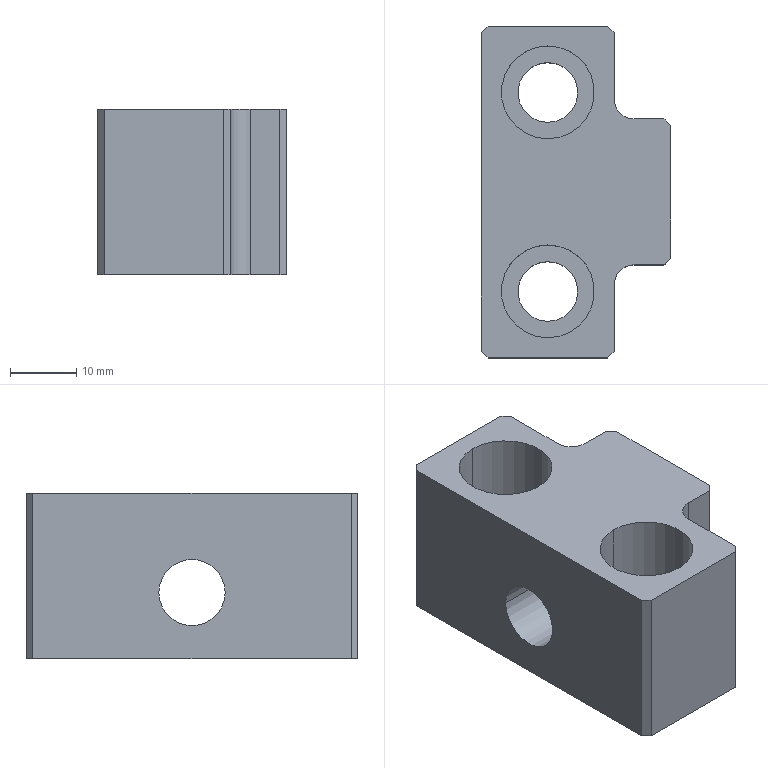Part | STEP file | J454-EBZ05-30-00-Part-1 | 1 solid | 30 faces | box 28.5 x 50 x 25 mm | volume 22471 mm3 | plane 18 | cylinder 12 | commonest cylinder face diameters 9 x4 14 x4 6 x2 10 x2
STEP:
#1=CARTESIAN_POINT('',(18.5,-5.,0.));
#2=VERTEX_POINT('',#1);
#3=CARTESIAN_POINT('',(18.5,5.,0.));
#4=VERTEX_POINT('',#3);
#5=CARTESIAN_POINT('',(18.5,0.,0.));
#6=DIRECTION('',(-1.,0.,0.));
#7=DIRECTION('',(0.,1.,0.));
#8=AXIS2_PLACEMENT_3D('',#5,#6,#7);
#9=CIRCLE('',#8,5.);
#10=EDGE_CURVE('',#2,#4,#9,.T.);
#11=ORIENTED_EDGE('',*,*,#10,.F.);
#12=CARTESIAN_POINT('',(-10.,-5.,0.));
#13=VERTEX_POINT('',#12);
#14=CARTESIAN_POINT('',(18.5,-5.,0.));
#15=DIRECTION('',(-1.,0.,0.));
#16=VECTOR('',#15,1000.);
#17=LINE('',#14,#16);
#18=EDGE_CURVE('',#2,#13,#17,.T.);
#19=ORIENTED_EDGE('',*,*,#18,.T.);
#20=CARTESIAN_POINT('',(-10.,5.,0.));
#21=VERTEX_POINT('',#20);
#22=CARTESIAN_POINT('',(-10.,0.,0.));
#23=DIRECTION('',(1.,0.,0.));
#24=DIRECTION('',(0.,-1.,0.));
#25=AXIS2_PLACEMENT_3D('',#22,#23,#24);
#26=CIRCLE('',#25,5.);
#27=EDGE_CURVE('',#21,#13,#26,.T.);
#28=ORIENTED_EDGE('',*,*,#27,.F.);
#29=CARTESIAN_POINT('',(18.5,5.,0.));
#30=DIRECTION('',(-1.,0.,0.));
#31=VECTOR('',#30,1000.);
#32=LINE('',#29,#31);
#33=EDGE_CURVE('',#4,#21,#32,.T.);
#34=ORIENTED_EDGE('',*,*,#33,.F.);
#35=EDGE_LOOP('',(#11,#19,#28,#34));
#36=FACE_OUTER_BOUND('',#35,.T.);
#37=CARTESIAN_POINT('',(18.5,0.,0.));
#38=DIRECTION('',(-1.,0.,0.));
#39=DIRECTION('',(0.,1.,0.));
#40=AXIS2_PLACEMENT_3D('',#37,#38,#39);
#41=CYLINDRICAL_SURFACE('',#40,5.);
#42=ADVANCED_FACE('',(#36),#41,.F.);
#43=CARTESIAN_POINT('',(0.,19.5,-10.));
#44=VERTEX_POINT('',#43);
#45=CARTESIAN_POINT('',(0.,10.5,-10.));
#46=VERTEX_POINT('',#45);
#47=CARTESIAN_POINT('',(0.,15.,-10.));
#48=DIRECTION('',(0.,0.,1.));
#49=DIRECTION('',(0.,-1.,0.));
#50=AXIS2_PLACEMENT_3D('',#47,#48,#49);
#51=CIRCLE('',#50,4.5);
#52=EDGE_CURVE('',#44,#46,#51,.T.);
#53=ORIENTED_EDGE('',*,*,#52,.F.);
#54=CARTESIAN_POINT('',(0.,19.5,5.));
#55=VERTEX_POINT('',#54);
#56=CARTESIAN_POINT('',(0.,19.5,15.));
#57=DIRECTION('',(0.,0.,1.));
#58=VECTOR('',#57,1000.);
#59=LINE('',#56,#58);
#60=EDGE_CURVE('',#44,#55,#59,.T.);
#61=ORIENTED_EDGE('',*,*,#60,.T.);
#62=CARTESIAN_POINT('',(0.,10.5,5.));
#63=VERTEX_POINT('',#62);
#64=CARTESIAN_POINT('',(0.,15.,5.));
#65=DIRECTION('',(0.,0.,1.));
#66=DIRECTION('',(0.,-1.,0.));
#67=AXIS2_PLACEMENT_3D('',#64,#65,#66);
#68=CIRCLE('',#67,4.5);
#69=EDGE_CURVE('',#55,#63,#68,.T.);
#70=ORIENTED_EDGE('',*,*,#69,.T.);
#71=CARTESIAN_POINT('',(0.,10.5,15.));
#72=DIRECTION('',(0.,0.,1.));
#73=VECTOR('',#72,1000.);
#74=LINE('',#71,#73);
#75=EDGE_CURVE('',#46,#63,#74,.T.);
#76=ORIENTED_EDGE('',*,*,#75,.F.);
#77=EDGE_LOOP('',(#53,#61,#70,#76));
#78=FACE_OUTER_BOUND('',#77,.T.);
#79=CARTESIAN_POINT('',(0.,15.,15.));
#80=DIRECTION('',(0.,0.,1.));
#81=DIRECTION('',(0.,-1.,0.));
#82=AXIS2_PLACEMENT_3D('',#79,#80,#81);
#83=CYLINDRICAL_SURFACE('',#82,4.5);
#84=ADVANCED_FACE('',(#78),#83,.F.);
#85=CARTESIAN_POINT('',(0.,22.,5.));
#86=VERTEX_POINT('',#85);
#87=CARTESIAN_POINT('',(0.,8.,5.));
#88=VERTEX_POINT('',#87);
#89=CARTESIAN_POINT('',(0.,15.,5.));
#90=DIRECTION('',(0.,0.,1.));
#91=DIRECTION('',(0.,-1.,0.));
#92=AXIS2_PLACEMENT_3D('',#89,#90,#91);
#93=CIRCLE('',#92,7.);
#94=EDGE_CURVE('',#86,#88,#93,.T.);
#95=ORIENTED_EDGE('',*,*,#94,.F.);
#96=CARTESIAN_POINT('',(0.,22.,15.));
#97=VERTEX_POINT('',#96);
#98=CARTESIAN_POINT('',(0.,22.,15.));
#99=DIRECTION('',(0.,0.,1.));
#100=VECTOR('',#99,1000.);
#101=LINE('',#98,#100);
#102=EDGE_CURVE('',#86,#97,#101,.T.);
#103=ORIENTED_EDGE('',*,*,#102,.T.);
#104=CARTESIAN_POINT('',(0.,8.,15.));
#105=VERTEX_POINT('',#104);
#106=CARTESIAN_POINT('',(0.,15.,15.));
#107=DIRECTION('',(0.,0.,1.));
#108=DIRECTION('',(0.,-1.,0.));
#109=AXIS2_PLACEMENT_3D('',#106,#107,#108);
#110=CIRCLE('',#109,7.);
#111=EDGE_CURVE('',#97,#105,#110,.T.);
#112=ORIENTED_EDGE('',*,*,#111,.T.);
#113=CARTESIAN_POINT('',(0.,8.,15.));
#114=DIRECTION('',(0.,0.,1.));
#115=VECTOR('',#114,1000.);
#116=LINE('',#113,#115);
#117=EDGE_CURVE('',#88,#105,#116,.T.);
#118=ORIENTED_EDGE('',*,*,#117,.F.);
#119=EDGE_LOOP('',(#95,#103,#112,#118));
#120=FACE_OUTER_BOUND('',#119,.T.);
#121=CARTESIAN_POINT('',(0.,15.,15.));
#122=DIRECTION('',(0.,0.,1.));
#123=DIRECTION('',(0.,-1.,0.));
#124=AXIS2_PLACEMENT_3D('',#121,#122,#123);
#125=CYLINDRICAL_SURFACE('',#124,7.);
#126=ADVANCED_FACE('',(#120),#125,.F.);
#127=CARTESIAN_POINT('',(0.,-10.5,-10.));
#128=VERTEX_POINT('',#127);
#129=CARTESIAN_POINT('',(0.,-19.5,-10.));
#130=VERTEX_POINT('',#129);
#131=CARTESIAN_POINT('',(0.,-15.,-10.));
#132=DIRECTION('',(0.,0.,1.));
#133=DIRECTION('',(0.,-1.,0.));
#134=AXIS2_PLACEMENT_3D('',#131,#132,#133);
#135=CIRCLE('',#134,4.5);
#136=EDGE_CURVE('',#128,#130,#135,.T.);
#137=ORIENTED_EDGE('',*,*,#136,.F.);
#138=CARTESIAN_POINT('',(0.,-10.5,5.));
#139=VERTEX_POINT('',#138);
#140=CARTESIAN_POINT('',(0.,-10.5,15.));
#141=DIRECTION('',(0.,0.,1.));
#142=VECTOR('',#141,1000.);
#143=LINE('',#140,#142);
#144=EDGE_CURVE('',#128,#139,#143,.T.);
#145=ORIENTED_EDGE('',*,*,#144,.T.);
#146=CARTESIAN_POINT('',(0.,-19.5,5.));
#147=VERTEX_POINT('',#146);
#148=CARTESIAN_POINT('',(0.,-15.,5.));
#149=DIRECTION('',(0.,0.,1.));
#150=DIRECTION('',(0.,-1.,0.));
#151=AXIS2_PLACEMENT_3D('',#148,#149,#150);
#152=CIRCLE('',#151,4.5);
#153=EDGE_CURVE('',#139,#147,#152,.T.);
#154=ORIENTED_EDGE('',*,*,#153,.T.);
#155=CARTESIAN_POINT('',(0.,-19.5,15.));
#156=DIRECTION('',(0.,0.,1.));
#157=VECTOR('',#156,1000.);
#158=LINE('',#155,#157);
#159=EDGE_CURVE('',#130,#147,#158,.T.);
#160=ORIENTED_EDGE('',*,*,#159,.F.);
#161=EDGE_LOOP('',(#137,#145,#154,#160));
#162=FACE_OUTER_BOUND('',#161,.T.);
#163=CARTESIAN_POINT('',(0.,-15.,15.));
#164=DIRECTION('',(0.,0.,1.));
#165=DIRECTION('',(0.,-1.,0.));
#166=AXIS2_PLACEMENT_3D('',#163,#164,#165);
#167=CYLINDRICAL_SURFACE('',#166,4.5);
#168=ADVANCED_FACE('',(#162),#167,.F.);
#169=CARTESIAN_POINT('',(0.,-8.,5.));
#170=VERTEX_POINT('',#169);
#171=CARTESIAN_POINT('',(0.,-22.,5.));
#172=VERTEX_POINT('',#171);
#173=CARTESIAN_POINT('',(0.,-15.,5.));
#174=DIRECTION('',(0.,0.,1.));
#175=DIRECTION('',(0.,-1.,0.));
#176=AXIS2_PLACEMENT_3D('',#173,#174,#175);
#177=CIRCLE('',#176,7.);
#178=EDGE_CURVE('',#170,#172,#177,.T.);
#179=ORIENTED_EDGE('',*,*,#178,.F.);
#180=CARTESIAN_POINT('',(0.,-8.,15.));
#181=VERTEX_POINT('',#180);
#182=CARTESIAN_POINT('',(0.,-8.,15.));
#183=DIRECTION('',(0.,0.,1.));
#184=VECTOR('',#183,1000.);
#185=LINE('',#182,#184);
#186=EDGE_CURVE('',#170,#181,#185,.T.);
#187=ORIENTED_EDGE('',*,*,#186,.T.);
#188=CARTESIAN_POINT('',(0.,-22.,15.));
#189=VERTEX_POINT('',#188);
#190=CARTESIAN_POINT('',(0.,-15.,15.));
#191=DIRECTION('',(0.,0.,1.));
#192=DIRECTION('',(0.,-1.,0.));
#193=AXIS2_PLACEMENT_3D('',#190,#191,#192);
#194=CIRCLE('',#193,7.);
#195=EDGE_CURVE('',#181,#189,#194,.T.);
#196=ORIENTED_EDGE('',*,*,#195,.T.);
#197=CARTESIAN_POINT('',(0.,-22.,15.));
#198=DIRECTION('',(0.,0.,1.));
#199=VECTOR('',#198,1000.);
#200=LINE('',#197,#199);
#201=EDGE_CURVE('',#172,#189,#200,.T.);
#202=ORIENTED_EDGE('',*,*,#201,.F.);
#203=EDGE_LOOP('',(#179,#187,#196,#202));
#204=FACE_OUTER_BOUND('',#203,.T.);
#205=CARTESIAN_POINT('',(0.,-15.,15.));
#206=DIRECTION('',(0.,0.,1.));
#207=DIRECTION('',(0.,-1.,0.));
#208=AXIS2_PLACEMENT_3D('',#205,#206,#207);
#209=CYLINDRICAL_SURFACE('',#208,7.);
#210=ADVANCED_FACE('',(#204),#209,.F.);
#211=CARTESIAN_POINT('',(10.,-14.,-10.));
#212=VERTEX_POINT('',#211);
#213=CARTESIAN_POINT('',(10.,-24.,-10.));
#214=VERTEX_POINT('',#213);
#215=CARTESIAN_POINT('',(10.,24.,-10.));
#216=DIRECTION('',(0.,-1.,0.));
#217=VECTOR('',#216,1000.);
#218=LINE('',#215,#217);
#219=EDGE_CURVE('',#212,#214,#218,.T.);
#220=ORIENTED_EDGE('',*,*,#219,.F.);
#221=CARTESIAN_POINT('',(10.,-14.,15.));
#222=VERTEX_POINT('',#221);
#223=CARTESIAN_POINT('',(10.,-14.,15.));
#224=DIRECTION('',(0.,0.,1.));
#225=VECTOR('',#224,1000.);
#226=LINE('',#223,#225);
#227=EDGE_CURVE('',#212,#222,#226,.T.);
#228=ORIENTED_EDGE('',*,*,#227,.T.);
#229=CARTESIAN_POINT('',(10.,-24.,15.));
#230=VERTEX_POINT('',#229);
#231=CARTESIAN_POINT('',(10.,24.,15.));
#232=DIRECTION('',(0.,-1.,0.));
#233=VECTOR('',#232,1000.);
#234=LINE('',#231,#233);
#235=EDGE_CURVE('',#222,#230,#234,.T.);
#236=ORIENTED_EDGE('',*,*,#235,.T.);
#237=CARTESIAN_POINT('',(10.,-24.,13.));
#238=DIRECTION('',(0.,0.,-1.));
#239=VECTOR('',#238,1000.);
#240=LINE('',#237,#239);
#241=EDGE_CURVE('',#230,#214,#240,.T.);
#242=ORIENTED_EDGE('',*,*,#241,.T.);
#243=EDGE_LOOP('',(#220,#228,#236,#242));
#244=FACE_OUTER_BOUND('',#243,.T.);
#245=CARTESIAN_POINT('',(10.,39.919,41.419));
#246=DIRECTION('',(1.,0.,0.));
#247=DIRECTION('',(0.,0.,-1.));
#248=AXIS2_PLACEMENT_3D('',#245,#246,#247);
#249=PLANE('',#248);
#250=ADVANCED_FACE('',(#244),#249,.T.);
#251=CARTESIAN_POINT('',(9.,25.,-10.));
#252=VERTEX_POINT('',#251);
#253=CARTESIAN_POINT('',(-9.,25.,-10.));
#254=VERTEX_POINT('',#253);
#255=CARTESIAN_POINT('',(9.,25.,-10.));
#256=DIRECTION('',(-1.,0.,0.));
#257=VECTOR('',#256,1000.);
#258=LINE('',#255,#257);
#259=EDGE_CURVE('',#252,#254,#258,.T.);
#260=ORIENTED_EDGE('',*,*,#259,.T.);
#261=CARTESIAN_POINT('',(-9.,25.,15.));
#262=VERTEX_POINT('',#261);
#263=CARTESIAN_POINT('',(-9.,25.,13.));
#264=DIRECTION('',(0.,0.,-1.));
#265=VECTOR('',#264,1000.);
#266=LINE('',#263,#265);
#267=EDGE_CURVE('',#262,#254,#266,.T.);
#268=ORIENTED_EDGE('',*,*,#267,.F.);
#269=CARTESIAN_POINT('',(9.,25.,15.));
#270=VERTEX_POINT('',#269);
#271=CARTESIAN_POINT('',(-9.,25.,15.));
#272=DIRECTION('',(1.,0.,0.));
#273=VECTOR('',#272,1000.);
#274=LINE('',#271,#273);
#275=EDGE_CURVE('',#262,#270,#274,.T.);
#276=ORIENTED_EDGE('',*,*,#275,.T.);
#277=CARTESIAN_POINT('',(9.,25.,-10.));
#278=DIRECTION('',(0.,0.,1.));
#279=VECTOR('',#278,1000.);
#280=LINE('',#277,#279);
#281=EDGE_CURVE('',#252,#270,#280,.T.);
#282=ORIENTED_EDGE('',*,*,#281,.F.);
#283=EDGE_LOOP('',(#260,#268,#276,#282));
#284=FACE_OUTER_BOUND('',#283,.T.);
#285=CARTESIAN_POINT('',(21.905,25.,-20.405));
#286=DIRECTION('',(0.,-1.,0.));
#287=DIRECTION('',(-1.,0.,0.));
#288=AXIS2_PLACEMENT_3D('',#285,#286,#287);
#289=PLANE('',#288);
#290=ADVANCED_FACE('',(#284),#289,.F.);
#291=ORIENTED_EDGE('',*,*,#267,.T.);
#292=CARTESIAN_POINT('',(-10.,24.,-10.));
#293=VERTEX_POINT('',#292);
#294=CARTESIAN_POINT('',(-9.,25.,-10.));
#295=DIRECTION('',(-0.7071,-0.7071,0.));
#296=VECTOR('',#295,1000.);
#297=LINE('',#294,#296);
#298=EDGE_CURVE('',#254,#293,#297,.T.);
#299=ORIENTED_EDGE('',*,*,#298,.T.);
#300=CARTESIAN_POINT('',(-10.,24.,15.));
#301=VERTEX_POINT('',#300);
#302=CARTESIAN_POINT('',(-10.,24.,13.));
#303=DIRECTION('',(0.,0.,-1.));
#304=VECTOR('',#303,1000.);
#305=LINE('',#302,#304);
#306=EDGE_CURVE('',#301,#293,#305,.T.);
#307=ORIENTED_EDGE('',*,*,#306,.F.);
#308=CARTESIAN_POINT('',(-10.,24.,15.));
#309=DIRECTION('',(0.7071,0.7071,0.));
#310=VECTOR('',#309,1000.);
#311=LINE('',#308,#310);
#312=EDGE_CURVE('',#301,#262,#311,.T.);
#313=ORIENTED_EDGE('',*,*,#312,.T.);
#314=EDGE_LOOP('',(#291,#299,#307,#313));
#315=FACE_OUTER_BOUND('',#314,.T.);
#316=CARTESIAN_POINT('',(2.721,36.721,18.783));
#317=DIRECTION('',(-0.7071,0.7071,0.));
#318=DIRECTION('',(-0.7071,-0.7071,0.));
#319=AXIS2_PLACEMENT_3D('',#316,#317,#318);
#320=PLANE('',#319);
#321=ADVANCED_FACE('',(#315),#320,.T.);
#322=CARTESIAN_POINT('',(0.,15.,-10.));
#323=DIRECTION('',(0.,0.,1.));
#324=DIRECTION('',(0.,-1.,0.));
#325=AXIS2_PLACEMENT_3D('',#322,#323,#324);
#326=CIRCLE('',#325,4.5);
#327=EDGE_CURVE('',#46,#44,#326,.T.);
#328=ORIENTED_EDGE('',*,*,#327,.T.);
#329=ORIENTED_EDGE('',*,*,#52,.T.);
#330=EDGE_LOOP('',(#328,#329));
#331=FACE_BOUND('',#330,.T.);
#332=CARTESIAN_POINT('',(0.,-15.,-10.));
#333=DIRECTION('',(0.,0.,1.));
#334=DIRECTION('',(0.,-1.,0.));
#335=AXIS2_PLACEMENT_3D('',#332,#333,#334);
#336=CIRCLE('',#335,4.5);
#337=EDGE_CURVE('',#130,#128,#336,.T.);
#338=ORIENTED_EDGE('',*,*,#337,.T.);
#339=ORIENTED_EDGE('',*,*,#136,.T.);
#340=EDGE_LOOP('',(#338,#339));
#341=FACE_BOUND('',#340,.T.);
#342=CARTESIAN_POINT('',(13.,11.,-10.));
#343=VERTEX_POINT('',#342);
#344=CARTESIAN_POINT('',(17.5,11.,-10.));
#345=VERTEX_POINT('',#344);
#346=CARTESIAN_POINT('',(10.,11.,-10.));
#347=DIRECTION('',(1.,0.,0.));
#348=VECTOR('',#347,1000.);
#349=LINE('',#346,#348);
#350=EDGE_CURVE('',#343,#345,#349,.T.);
#351=ORIENTED_EDGE('',*,*,#350,.T.);
#352=CARTESIAN_POINT('',(18.5,10.,-10.));
#353=VERTEX_POINT('',#352);
#354=CARTESIAN_POINT('',(14.25,14.25,-10.));
#355=DIRECTION('',(0.7071,-0.7071,0.));
#356=VECTOR('',#355,1000.);
#357=LINE('',#354,#356);
#358=EDGE_CURVE('',#345,#353,#357,.T.);
#359=ORIENTED_EDGE('',*,*,#358,.T.);
#360=CARTESIAN_POINT('',(18.5,-10.,-10.));
#361=VERTEX_POINT('',#360);
#362=CARTESIAN_POINT('',(18.5,0.,-10.));
#363=DIRECTION('',(0.,-1.,0.));
#364=VECTOR('',#363,1000.);
#365=LINE('',#362,#364);
#366=EDGE_CURVE('',#353,#361,#365,.T.);
#367=ORIENTED_EDGE('',*,*,#366,.T.);
#368=CARTESIAN_POINT('',(17.5,-11.,-10.));
#369=VERTEX_POINT('',#368);
#370=CARTESIAN_POINT('',(54.639,26.139,-10.));
#371=DIRECTION('',(-0.7071,-0.7071,0.));
#372=VECTOR('',#371,1000.);
#373=LINE('',#370,#372);
#374=EDGE_CURVE('',#361,#369,#373,.T.);
#375=ORIENTED_EDGE('',*,*,#374,.T.);
#376=CARTESIAN_POINT('',(13.,-11.,-10.));
#377=VERTEX_POINT('',#376);
#378=CARTESIAN_POINT('',(10.,-11.,-10.));
#379=DIRECTION('',(1.,0.,0.));
#380=VECTOR('',#379,1000.);
#381=LINE('',#378,#380);
#382=EDGE_CURVE('',#377,#369,#381,.T.);
#383=ORIENTED_EDGE('',*,*,#382,.F.);
#384=CARTESIAN_POINT('',(13.,-14.,-10.));
#385=DIRECTION('',(0.,0.,1.));
#386=DIRECTION('',(1.,0.,0.));
#387=AXIS2_PLACEMENT_3D('',#384,#385,#386);
#388=CIRCLE('',#387,3.);
#389=EDGE_CURVE('',#377,#212,#388,.T.);
#390=ORIENTED_EDGE('',*,*,#389,.T.);
#391=ORIENTED_EDGE('',*,*,#219,.T.);
#392=CARTESIAN_POINT('',(9.,-25.,-10.));
#393=VERTEX_POINT('',#392);
#394=CARTESIAN_POINT('',(9.,-25.,-10.));
#395=DIRECTION('',(0.7071,0.7071,0.));
#396=VECTOR('',#395,1000.);
#397=LINE('',#394,#396);
#398=EDGE_CURVE('',#393,#214,#397,.T.);
#399=ORIENTED_EDGE('',*,*,#398,.F.);
#400=CARTESIAN_POINT('',(-9.,-25.,-10.));
#401=VERTEX_POINT('',#400);
#402=CARTESIAN_POINT('',(9.,-25.,-10.));
#403=DIRECTION('',(-1.,0.,0.));
#404=VECTOR('',#403,1000.);
#405=LINE('',#402,#404);
#406=EDGE_CURVE('',#393,#401,#405,.T.);
#407=ORIENTED_EDGE('',*,*,#406,.T.);
#408=CARTESIAN_POINT('',(-10.,-24.,-10.));
#409=VERTEX_POINT('',#408);
#410=CARTESIAN_POINT('',(-10.,-24.,-10.));
#411=DIRECTION('',(0.7071,-0.7071,0.));
#412=VECTOR('',#411,1000.);
#413=LINE('',#410,#412);
#414=EDGE_CURVE('',#409,#401,#413,.T.);
#415=ORIENTED_EDGE('',*,*,#414,.F.);
#416=CARTESIAN_POINT('',(-10.,24.,-10.));
#417=DIRECTION('',(0.,-1.,0.));
#418=VECTOR('',#417,1000.);
#419=LINE('',#416,#418);
#420=EDGE_CURVE('',#293,#409,#419,.T.);
#421=ORIENTED_EDGE('',*,*,#420,.F.);
#422=ORIENTED_EDGE('',*,*,#298,.F.);
#423=ORIENTED_EDGE('',*,*,#259,.F.);
#424=CARTESIAN_POINT('',(10.,24.,-10.));
#425=VERTEX_POINT('',#424);
#426=CARTESIAN_POINT('',(10.,24.,-10.));
#427=DIRECTION('',(-0.7071,0.7071,0.));
#428=VECTOR('',#427,1000.);
#429=LINE('',#426,#428);
#430=EDGE_CURVE('',#425,#252,#429,.T.);
#431=ORIENTED_EDGE('',*,*,#430,.F.);
#432=CARTESIAN_POINT('',(10.,14.,-10.));
#433=VERTEX_POINT('',#432);
#434=CARTESIAN_POINT('',(10.,24.,-10.));
#435=DIRECTION('',(0.,-1.,0.));
#436=VECTOR('',#435,1000.);
#437=LINE('',#434,#436);
#438=EDGE_CURVE('',#425,#433,#437,.T.);
#439=ORIENTED_EDGE('',*,*,#438,.T.);
#440=CARTESIAN_POINT('',(13.,14.,-10.));
#441=DIRECTION('',(0.,0.,1.));
#442=DIRECTION('',(1.,0.,0.));
#443=AXIS2_PLACEMENT_3D('',#440,#441,#442);
#444=CIRCLE('',#443,3.);
#445=EDGE_CURVE('',#433,#343,#444,.T.);
#446=ORIENTED_EDGE('',*,*,#445,.T.);
#447=EDGE_LOOP('',(#351,#359,#367,#375,#383,#390,#391,#399,#407,#415,#421,#422,#423,#431,#439,#446));
#448=FACE_OUTER_BOUND('',#447,.T.);
#449=CARTESIAN_POINT('',(40.389,40.389,-10.));
#450=DIRECTION('',(0.,0.,-1.));
#451=DIRECTION('',(-1.,0.,0.));
#452=AXIS2_PLACEMENT_3D('',#449,#450,#451);
#453=PLANE('',#452);
#454=ADVANCED_FACE('',(#331,#341,#448),#453,.T.);
#455=CARTESIAN_POINT('',(0.,15.,15.));
#456=DIRECTION('',(0.,0.,1.));
#457=DIRECTION('',(0.,-1.,0.));
#458=AXIS2_PLACEMENT_3D('',#455,#456,#457);
#459=CIRCLE('',#458,7.);
#460=EDGE_CURVE('',#105,#97,#459,.T.);
#461=ORIENTED_EDGE('',*,*,#460,.F.);
#462=ORIENTED_EDGE('',*,*,#111,.F.);
#463=EDGE_LOOP('',(#461,#462));
#464=FACE_BOUND('',#463,.T.);
#465=CARTESIAN_POINT('',(0.,-15.,15.));
#466=DIRECTION('',(0.,0.,1.));
#467=DIRECTION('',(0.,-1.,0.));
#468=AXIS2_PLACEMENT_3D('',#465,#466,#467);
#469=CIRCLE('',#468,7.);
#470=EDGE_CURVE('',#189,#181,#469,.T.);
#471=ORIENTED_EDGE('',*,*,#470,.F.);
#472=ORIENTED_EDGE('',*,*,#195,.F.);
#473=EDGE_LOOP('',(#471,#472));
#474=FACE_BOUND('',#473,.T.);
#475=CARTESIAN_POINT('',(18.5,-10.,15.));
#476=VERTEX_POINT('',#475);
#477=CARTESIAN_POINT('',(18.5,10.,15.));
#478=VERTEX_POINT('',#477);
#479=CARTESIAN_POINT('',(18.5,0.,15.));
#480=DIRECTION('',(0.,1.,0.));
#481=VECTOR('',#480,1000.);
#482=LINE('',#479,#481);
#483=EDGE_CURVE('',#476,#478,#482,.T.);
#484=ORIENTED_EDGE('',*,*,#483,.T.);
#485=CARTESIAN_POINT('',(17.5,11.,15.));
#486=VERTEX_POINT('',#485);
#487=CARTESIAN_POINT('',(-26.139,54.639,15.));
#488=DIRECTION('',(-0.7071,0.7071,0.));
#489=VECTOR('',#488,1000.);
#490=LINE('',#487,#489);
#491=EDGE_CURVE('',#478,#486,#490,.T.);
#492=ORIENTED_EDGE('',*,*,#491,.T.);
#493=CARTESIAN_POINT('',(13.,11.,15.));
#494=VERTEX_POINT('',#493);
#495=CARTESIAN_POINT('',(10.,11.,15.));
#496=DIRECTION('',(1.,0.,0.));
#497=VECTOR('',#496,1000.);
#498=LINE('',#495,#497);
#499=EDGE_CURVE('',#494,#486,#498,.T.);
#500=ORIENTED_EDGE('',*,*,#499,.F.);
#501=CARTESIAN_POINT('',(10.,14.,15.));
#502=VERTEX_POINT('',#501);
#503=CARTESIAN_POINT('',(13.,14.,15.));
#504=DIRECTION('',(0.,0.,-1.));
#505=DIRECTION('',(-1.,0.,0.));
#506=AXIS2_PLACEMENT_3D('',#503,#504,#505);
#507=CIRCLE('',#506,3.);
#508=EDGE_CURVE('',#494,#502,#507,.T.);
#509=ORIENTED_EDGE('',*,*,#508,.T.);
#510=CARTESIAN_POINT('',(10.,24.,15.));
#511=VERTEX_POINT('',#510);
#512=CARTESIAN_POINT('',(10.,24.,15.));
#513=DIRECTION('',(0.,-1.,0.));
#514=VECTOR('',#513,1000.);
#515=LINE('',#512,#514);
#516=EDGE_CURVE('',#511,#502,#515,.T.);
#517=ORIENTED_EDGE('',*,*,#516,.F.);
#518=CARTESIAN_POINT('',(9.,25.,15.));
#519=DIRECTION('',(0.7071,-0.7071,0.));
#520=VECTOR('',#519,1000.);
#521=LINE('',#518,#520);
#522=EDGE_CURVE('',#270,#511,#521,.T.);
#523=ORIENTED_EDGE('',*,*,#522,.F.);
#524=ORIENTED_EDGE('',*,*,#275,.F.);
#525=ORIENTED_EDGE('',*,*,#312,.F.);
#526=CARTESIAN_POINT('',(-10.,-24.,15.));
#527=VERTEX_POINT('',#526);
#528=CARTESIAN_POINT('',(-10.,24.,15.));
#529=DIRECTION('',(0.,-1.,0.));
#530=VECTOR('',#529,1000.);
#531=LINE('',#528,#530);
#532=EDGE_CURVE('',#301,#527,#531,.T.);
#533=ORIENTED_EDGE('',*,*,#532,.T.);
#534=CARTESIAN_POINT('',(-9.,-25.,15.));
#535=VERTEX_POINT('',#534);
#536=CARTESIAN_POINT('',(-9.,-25.,15.));
#537=DIRECTION('',(-0.7071,0.7071,0.));
#538=VECTOR('',#537,1000.);
#539=LINE('',#536,#538);
#540=EDGE_CURVE('',#535,#527,#539,.T.);
#541=ORIENTED_EDGE('',*,*,#540,.F.);
#542=CARTESIAN_POINT('',(9.,-25.,15.));
#543=VERTEX_POINT('',#542);
#544=CARTESIAN_POINT('',(-9.,-25.,15.));
#545=DIRECTION('',(1.,0.,0.));
#546=VECTOR('',#545,1000.);
#547=LINE('',#544,#546);
#548=EDGE_CURVE('',#535,#543,#547,.T.);
#549=ORIENTED_EDGE('',*,*,#548,.T.);
#550=CARTESIAN_POINT('',(10.,-24.,15.));
#551=DIRECTION('',(-0.7071,-0.7071,0.));
#552=VECTOR('',#551,1000.);
#553=LINE('',#550,#552);
#554=EDGE_CURVE('',#230,#543,#553,.T.);
#555=ORIENTED_EDGE('',*,*,#554,.F.);
#556=ORIENTED_EDGE('',*,*,#235,.F.);
#557=CARTESIAN_POINT('',(13.,-11.,15.));
#558=VERTEX_POINT('',#557);
#559=CARTESIAN_POINT('',(13.,-14.,15.));
#560=DIRECTION('',(0.,0.,-1.));
#561=DIRECTION('',(-1.,0.,0.));
#562=AXIS2_PLACEMENT_3D('',#559,#560,#561);
#563=CIRCLE('',#562,3.);
#564=EDGE_CURVE('',#222,#558,#563,.T.);
#565=ORIENTED_EDGE('',*,*,#564,.T.);
#566=CARTESIAN_POINT('',(17.5,-11.,15.));
#567=VERTEX_POINT('',#566);
#568=CARTESIAN_POINT('',(10.,-11.,15.));
#569=DIRECTION('',(1.,0.,0.));
#570=VECTOR('',#569,1000.);
#571=LINE('',#568,#570);
#572=EDGE_CURVE('',#558,#567,#571,.T.);
#573=ORIENTED_EDGE('',*,*,#572,.T.);
#574=CARTESIAN_POINT('',(14.25,-14.25,15.));
#575=DIRECTION('',(0.7071,0.7071,0.));
#576=VECTOR('',#575,1000.);
#577=LINE('',#574,#576);
#578=EDGE_CURVE('',#567,#476,#577,.T.);
#579=ORIENTED_EDGE('',*,*,#578,.T.);
#580=EDGE_LOOP('',(#484,#492,#500,#509,#517,#523,#524,#525,#533,#541,#549,#555,#556,#565,#573,#579));
#581=FACE_OUTER_BOUND('',#580,.T.);
#582=CARTESIAN_POINT('',(-40.389,40.389,15.));
#583=DIRECTION('',(0.,0.,1.));
#584=DIRECTION('',(1.,0.,0.));
#585=AXIS2_PLACEMENT_3D('',#582,#583,#584);
#586=PLANE('',#585);
#587=ADVANCED_FACE('',(#464,#474,#581),#586,.T.);
#588=CARTESIAN_POINT('',(9.,-25.,13.));
#589=DIRECTION('',(0.,0.,-1.));
#590=VECTOR('',#589,1000.);
#591=LINE('',#588,#590);
#592=EDGE_CURVE('',#543,#393,#591,.T.);
#593=ORIENTED_EDGE('',*,*,#592,.T.);
#594=ORIENTED_EDGE('',*,*,#398,.T.);
#595=ORIENTED_EDGE('',*,*,#241,.F.);
#596=ORIENTED_EDGE('',*,*,#554,.T.);
#597=EDGE_LOOP('',(#593,#594,#595,#596));
#598=FACE_OUTER_BOUND('',#597,.T.);
#599=CARTESIAN_POINT('',(-2.721,-36.721,18.783));
#600=DIRECTION('',(0.7071,-0.7071,0.));
#601=DIRECTION('',(0.7071,0.7071,0.));
#602=AXIS2_PLACEMENT_3D('',#599,#600,#601);
#603=PLANE('',#602);
#604=ADVANCED_FACE('',(#598),#603,.T.);
#605=ORIENTED_EDGE('',*,*,#516,.T.);
#606=CARTESIAN_POINT('',(10.,14.,-10.));
#607=DIRECTION('',(0.,0.,-1.));
#608=VECTOR('',#607,1000.);
#609=LINE('',#606,#608);
#610=EDGE_CURVE('',#502,#433,#609,.T.);
#611=ORIENTED_EDGE('',*,*,#610,.T.);
#612=ORIENTED_EDGE('',*,*,#438,.F.);
#613=CARTESIAN_POINT('',(10.,24.,-10.));
#614=DIRECTION('',(0.,0.,1.));
#615=VECTOR('',#614,1000.);
#616=LINE('',#613,#615);
#617=EDGE_CURVE('',#425,#511,#616,.T.);
#618=ORIENTED_EDGE('',*,*,#617,.T.);
#619=EDGE_LOOP('',(#605,#611,#612,#618));
#620=FACE_OUTER_BOUND('',#619,.T.);
#621=CARTESIAN_POINT('',(10.,39.919,41.419));
#622=DIRECTION('',(1.,0.,0.));
#623=DIRECTION('',(0.,0.,-1.));
#624=AXIS2_PLACEMENT_3D('',#621,#622,#623);
#625=PLANE('',#624);
#626=ADVANCED_FACE('',(#620),#625,.T.);
#627=ORIENTED_EDGE('',*,*,#27,.T.);
#628=CARTESIAN_POINT('',(-10.,0.,0.));
#629=DIRECTION('',(1.,0.,0.));
#630=DIRECTION('',(0.,-1.,0.));
#631=AXIS2_PLACEMENT_3D('',#628,#629,#630);
#632=CIRCLE('',#631,5.);
#633=EDGE_CURVE('',#13,#21,#632,.T.);
#634=ORIENTED_EDGE('',*,*,#633,.T.);
#635=EDGE_LOOP('',(#627,#634));
#636=FACE_BOUND('',#635,.T.);
#637=ORIENTED_EDGE('',*,*,#420,.T.);
#638=CARTESIAN_POINT('',(-10.,-24.,-10.));
#639=DIRECTION('',(0.,0.,1.));
#640=VECTOR('',#639,1000.);
#641=LINE('',#638,#640);
#642=EDGE_CURVE('',#409,#527,#641,.T.);
#643=ORIENTED_EDGE('',*,*,#642,.T.);
#644=ORIENTED_EDGE('',*,*,#532,.F.);
#645=ORIENTED_EDGE('',*,*,#306,.T.);
#646=EDGE_LOOP('',(#637,#643,#644,#645));
#647=FACE_OUTER_BOUND('',#646,.T.);
#648=CARTESIAN_POINT('',(-10.,39.919,-38.419));
#649=DIRECTION('',(-1.,0.,0.));
#650=DIRECTION('',(0.,0.,1.));
#651=AXIS2_PLACEMENT_3D('',#648,#649,#650);
#652=PLANE('',#651);
#653=ADVANCED_FACE('',(#636,#647),#652,.T.);
#654=CARTESIAN_POINT('',(-9.,-25.,-10.));
#655=DIRECTION('',(0.,0.,1.));
#656=VECTOR('',#655,1000.);
#657=LINE('',#654,#656);
#658=EDGE_CURVE('',#401,#535,#657,.T.);
#659=ORIENTED_EDGE('',*,*,#658,.T.);
#660=ORIENTED_EDGE('',*,*,#540,.T.);
#661=ORIENTED_EDGE('',*,*,#642,.F.);
#662=ORIENTED_EDGE('',*,*,#414,.T.);
#663=EDGE_LOOP('',(#659,#660,#661,#662));
#664=FACE_OUTER_BOUND('',#663,.T.);
#665=CARTESIAN_POINT('',(2.721,-36.721,-15.783));
#666=DIRECTION('',(-0.7071,-0.7071,0.));
#667=DIRECTION('',(-0.7071,0.7071,0.));
#668=AXIS2_PLACEMENT_3D('',#665,#666,#667);
#669=PLANE('',#668);
#670=ADVANCED_FACE('',(#664),#669,.T.);
#671=ORIENTED_EDGE('',*,*,#406,.F.);
#672=ORIENTED_EDGE('',*,*,#592,.F.);
#673=ORIENTED_EDGE('',*,*,#548,.F.);
#674=ORIENTED_EDGE('',*,*,#658,.F.);
#675=EDGE_LOOP('',(#671,#672,#673,#674));
#676=FACE_OUTER_BOUND('',#675,.T.);
#677=CARTESIAN_POINT('',(21.905,-25.,-20.405));
#678=DIRECTION('',(0.,-1.,0.));
#679=DIRECTION('',(-1.,0.,0.));
#680=AXIS2_PLACEMENT_3D('',#677,#678,#679);
#681=PLANE('',#680);
#682=ADVANCED_FACE('',(#676),#681,.T.);
#683=ORIENTED_EDGE('',*,*,#281,.T.);
#684=ORIENTED_EDGE('',*,*,#522,.T.);
#685=ORIENTED_EDGE('',*,*,#617,.F.);
#686=ORIENTED_EDGE('',*,*,#430,.T.);
#687=EDGE_LOOP('',(#683,#684,#685,#686));
#688=FACE_OUTER_BOUND('',#687,.T.);
#689=CARTESIAN_POINT('',(-2.721,36.721,-15.783));
#690=DIRECTION('',(0.7071,0.7071,0.));
#691=DIRECTION('',(0.7071,-0.7071,0.));
#692=AXIS2_PLACEMENT_3D('',#689,#690,#691);
#693=PLANE('',#692);
#694=ADVANCED_FACE('',(#688),#693,.T.);
#695=ORIENTED_EDGE('',*,*,#186,.F.);
#696=CARTESIAN_POINT('',(0.,-15.,5.));
#697=DIRECTION('',(0.,0.,1.));
#698=DIRECTION('',(0.,-1.,0.));
#699=AXIS2_PLACEMENT_3D('',#696,#697,#698);
#700=CIRCLE('',#699,7.);
#701=EDGE_CURVE('',#172,#170,#700,.T.);
#702=ORIENTED_EDGE('',*,*,#701,.F.);
#703=ORIENTED_EDGE('',*,*,#201,.T.);
#704=ORIENTED_EDGE('',*,*,#470,.T.);
#705=EDGE_LOOP('',(#695,#702,#703,#704));
#706=FACE_OUTER_BOUND('',#705,.T.);
#707=CARTESIAN_POINT('',(0.,-15.,15.));
#708=DIRECTION('',(0.,0.,1.));
#709=DIRECTION('',(0.,-1.,0.));
#710=AXIS2_PLACEMENT_3D('',#707,#708,#709);
#711=CYLINDRICAL_SURFACE('',#710,7.);
#712=ADVANCED_FACE('',(#706),#711,.F.);
#713=CARTESIAN_POINT('',(0.,-15.,5.));
#714=DIRECTION('',(0.,0.,1.));
#715=DIRECTION('',(0.,-1.,0.));
#716=AXIS2_PLACEMENT_3D('',#713,#714,#715);
#717=CIRCLE('',#716,4.5);
#718=EDGE_CURVE('',#147,#139,#717,.T.);
#719=ORIENTED_EDGE('',*,*,#718,.F.);
#720=ORIENTED_EDGE('',*,*,#153,.F.);
#721=EDGE_LOOP('',(#719,#720));
#722=FACE_BOUND('',#721,.T.);
#723=ORIENTED_EDGE('',*,*,#701,.T.);
#724=ORIENTED_EDGE('',*,*,#178,.T.);
#725=EDGE_LOOP('',(#723,#724));
#726=FACE_OUTER_BOUND('',#725,.T.);
#727=CARTESIAN_POINT('',(0.,-8.,5.));
#728=DIRECTION('',(0.,0.,-1.));
#729=DIRECTION('',(0.,1.,0.));
#730=AXIS2_PLACEMENT_3D('',#727,#728,#729);
#731=PLANE('',#730);
#732=ADVANCED_FACE('',(#722,#726),#731,.F.);
#733=ORIENTED_EDGE('',*,*,#144,.F.);
#734=ORIENTED_EDGE('',*,*,#337,.F.);
#735=ORIENTED_EDGE('',*,*,#159,.T.);
#736=ORIENTED_EDGE('',*,*,#718,.T.);
#737=EDGE_LOOP('',(#733,#734,#735,#736));
#738=FACE_OUTER_BOUND('',#737,.T.);
#739=CARTESIAN_POINT('',(0.,-15.,15.));
#740=DIRECTION('',(0.,0.,1.));
#741=DIRECTION('',(0.,-1.,0.));
#742=AXIS2_PLACEMENT_3D('',#739,#740,#741);
#743=CYLINDRICAL_SURFACE('',#742,4.5);
#744=ADVANCED_FACE('',(#738),#743,.F.);
#745=ORIENTED_EDGE('',*,*,#102,.F.);
#746=CARTESIAN_POINT('',(0.,15.,5.));
#747=DIRECTION('',(0.,0.,1.));
#748=DIRECTION('',(0.,-1.,0.));
#749=AXIS2_PLACEMENT_3D('',#746,#747,#748);
#750=CIRCLE('',#749,7.);
#751=EDGE_CURVE('',#88,#86,#750,.T.);
#752=ORIENTED_EDGE('',*,*,#751,.F.);
#753=ORIENTED_EDGE('',*,*,#117,.T.);
#754=ORIENTED_EDGE('',*,*,#460,.T.);
#755=EDGE_LOOP('',(#745,#752,#753,#754));
#756=FACE_OUTER_BOUND('',#755,.T.);
#757=CARTESIAN_POINT('',(0.,15.,15.));
#758=DIRECTION('',(0.,0.,1.));
#759=DIRECTION('',(0.,-1.,0.));
#760=AXIS2_PLACEMENT_3D('',#757,#758,#759);
#761=CYLINDRICAL_SURFACE('',#760,7.);
#762=ADVANCED_FACE('',(#756),#761,.F.);
#763=CARTESIAN_POINT('',(0.,15.,5.));
#764=DIRECTION('',(0.,0.,1.));
#765=DIRECTION('',(0.,-1.,0.));
#766=AXIS2_PLACEMENT_3D('',#763,#764,#765);
#767=CIRCLE('',#766,4.5);
#768=EDGE_CURVE('',#63,#55,#767,.T.);
#769=ORIENTED_EDGE('',*,*,#768,.F.);
#770=ORIENTED_EDGE('',*,*,#69,.F.);
#771=EDGE_LOOP('',(#769,#770));
#772=FACE_BOUND('',#771,.T.);
#773=ORIENTED_EDGE('',*,*,#751,.T.);
#774=ORIENTED_EDGE('',*,*,#94,.T.);
#775=EDGE_LOOP('',(#773,#774));
#776=FACE_OUTER_BOUND('',#775,.T.);
#777=CARTESIAN_POINT('',(0.,22.,5.));
#778=DIRECTION('',(0.,0.,-1.));
#779=DIRECTION('',(0.,1.,0.));
#780=AXIS2_PLACEMENT_3D('',#777,#778,#779);
#781=PLANE('',#780);
#782=ADVANCED_FACE('',(#772,#776),#781,.F.);
#783=ORIENTED_EDGE('',*,*,#60,.F.);
#784=ORIENTED_EDGE('',*,*,#327,.F.);
#785=ORIENTED_EDGE('',*,*,#75,.T.);
#786=ORIENTED_EDGE('',*,*,#768,.T.);
#787=EDGE_LOOP('',(#783,#784,#785,#786));
#788=FACE_OUTER_BOUND('',#787,.T.);
#789=CARTESIAN_POINT('',(0.,15.,15.));
#790=DIRECTION('',(0.,0.,1.));
#791=DIRECTION('',(0.,-1.,0.));
#792=AXIS2_PLACEMENT_3D('',#789,#790,#791);
#793=CYLINDRICAL_SURFACE('',#792,4.5);
#794=ADVANCED_FACE('',(#788),#793,.F.);
#795=CARTESIAN_POINT('',(18.5,0.,0.));
#796=DIRECTION('',(-1.,0.,0.));
#797=DIRECTION('',(0.,1.,0.));
#798=AXIS2_PLACEMENT_3D('',#795,#796,#797);
#799=CIRCLE('',#798,5.);
#800=EDGE_CURVE('',#4,#2,#799,.T.);
#801=ORIENTED_EDGE('',*,*,#800,.T.);
#802=ORIENTED_EDGE('',*,*,#10,.T.);
#803=EDGE_LOOP('',(#801,#802));
#804=FACE_BOUND('',#803,.T.);
#805=ORIENTED_EDGE('',*,*,#366,.F.);
#806=CARTESIAN_POINT('',(18.5,10.,2.5));
#807=DIRECTION('',(0.,0.,1.));
#808=VECTOR('',#807,1000.);
#809=LINE('',#806,#808);
#810=EDGE_CURVE('',#353,#478,#809,.T.);
#811=ORIENTED_EDGE('',*,*,#810,.T.);
#812=ORIENTED_EDGE('',*,*,#483,.F.);
#813=CARTESIAN_POINT('',(18.5,-10.,2.5));
#814=DIRECTION('',(0.,0.,-1.));
#815=VECTOR('',#814,1000.);
#816=LINE('',#813,#815);
#817=EDGE_CURVE('',#476,#361,#816,.T.);
#818=ORIENTED_EDGE('',*,*,#817,.T.);
#819=EDGE_LOOP('',(#805,#811,#812,#818));
#820=FACE_OUTER_BOUND('',#819,.T.);
#821=CARTESIAN_POINT('',(18.5,0.,2.5));
#822=DIRECTION('',(1.,0.,0.));
#823=DIRECTION('',(0.,-1.,0.));
#824=AXIS2_PLACEMENT_3D('',#821,#822,#823);
#825=PLANE('',#824);
#826=ADVANCED_FACE('',(#804,#820),#825,.T.);
#827=ORIENTED_EDGE('',*,*,#499,.T.);
#828=CARTESIAN_POINT('',(17.5,11.,2.5));
#829=DIRECTION('',(0.,0.,-1.));
#830=VECTOR('',#829,1000.);
#831=LINE('',#828,#830);
#832=EDGE_CURVE('',#486,#345,#831,.T.);
#833=ORIENTED_EDGE('',*,*,#832,.T.);
#834=ORIENTED_EDGE('',*,*,#350,.F.);
#835=CARTESIAN_POINT('',(13.,11.,15.));
#836=DIRECTION('',(0.,0.,1.));
#837=VECTOR('',#836,1000.);
#838=LINE('',#835,#837);
#839=EDGE_CURVE('',#343,#494,#838,.T.);
#840=ORIENTED_EDGE('',*,*,#839,.T.);
#841=EDGE_LOOP('',(#827,#833,#834,#840));
#842=FACE_OUTER_BOUND('',#841,.T.);
#843=CARTESIAN_POINT('',(10.,11.,2.5));
#844=DIRECTION('',(0.,1.,0.));
#845=DIRECTION('',(1.,0.,0.));
#846=AXIS2_PLACEMENT_3D('',#843,#844,#845);
#847=PLANE('',#846);
#848=ADVANCED_FACE('',(#842),#847,.T.);
#849=ORIENTED_EDGE('',*,*,#382,.T.);
#850=CARTESIAN_POINT('',(17.5,-11.,2.5));
#851=DIRECTION('',(0.,0.,1.));
#852=VECTOR('',#851,1000.);
#853=LINE('',#850,#852);
#854=EDGE_CURVE('',#369,#567,#853,.T.);
#855=ORIENTED_EDGE('',*,*,#854,.T.);
#856=ORIENTED_EDGE('',*,*,#572,.F.);
#857=CARTESIAN_POINT('',(13.,-11.,-10.));
#858=DIRECTION('',(0.,0.,-1.));
#859=VECTOR('',#858,1000.);
#860=LINE('',#857,#859);
#861=EDGE_CURVE('',#558,#377,#860,.T.);
#862=ORIENTED_EDGE('',*,*,#861,.T.);
#863=EDGE_LOOP('',(#849,#855,#856,#862));
#864=FACE_OUTER_BOUND('',#863,.T.);
#865=CARTESIAN_POINT('',(10.,-11.,2.5));
#866=DIRECTION('',(0.,-1.,0.));
#867=DIRECTION('',(-1.,0.,0.));
#868=AXIS2_PLACEMENT_3D('',#865,#866,#867);
#869=PLANE('',#868);
#870=ADVANCED_FACE('',(#864),#869,.T.);
#871=ORIENTED_EDGE('',*,*,#564,.F.);
#872=ORIENTED_EDGE('',*,*,#227,.F.);
#873=ORIENTED_EDGE('',*,*,#389,.F.);
#874=ORIENTED_EDGE('',*,*,#861,.F.);
#875=EDGE_LOOP('',(#871,#872,#873,#874));
#876=FACE_OUTER_BOUND('',#875,.T.);
#877=CARTESIAN_POINT('',(13.,-14.,2.5));
#878=DIRECTION('',(0.,0.,1.));
#879=DIRECTION('',(-1.,0.,0.));
#880=AXIS2_PLACEMENT_3D('',#877,#878,#879);
#881=CYLINDRICAL_SURFACE('',#880,3.);
#882=ADVANCED_FACE('',(#876),#881,.F.);
#883=ORIENTED_EDGE('',*,*,#445,.F.);
#884=ORIENTED_EDGE('',*,*,#610,.F.);
#885=ORIENTED_EDGE('',*,*,#508,.F.);
#886=ORIENTED_EDGE('',*,*,#839,.F.);
#887=EDGE_LOOP('',(#883,#884,#885,#886));
#888=FACE_OUTER_BOUND('',#887,.T.);
#889=CARTESIAN_POINT('',(13.,14.,2.5));
#890=DIRECTION('',(0.,0.,-1.));
#891=DIRECTION('',(1.,0.,0.));
#892=AXIS2_PLACEMENT_3D('',#889,#890,#891);
#893=CYLINDRICAL_SURFACE('',#892,3.);
#894=ADVANCED_FACE('',(#888),#893,.F.);
#895=ORIENTED_EDGE('',*,*,#374,.F.);
#896=ORIENTED_EDGE('',*,*,#817,.F.);
#897=ORIENTED_EDGE('',*,*,#578,.F.);
#898=ORIENTED_EDGE('',*,*,#854,.F.);
#899=EDGE_LOOP('',(#895,#896,#897,#898));
#900=FACE_OUTER_BOUND('',#899,.T.);
#901=CARTESIAN_POINT('',(17.5,-11.,2.5));
#902=DIRECTION('',(-0.7071,0.7071,0.));
#903=DIRECTION('',(0.,0.,1.));
#904=AXIS2_PLACEMENT_3D('',#901,#902,#903);
#905=PLANE('',#904);
#906=ADVANCED_FACE('',(#900),#905,.F.);
#907=ORIENTED_EDGE('',*,*,#491,.F.);
#908=ORIENTED_EDGE('',*,*,#810,.F.);
#909=ORIENTED_EDGE('',*,*,#358,.F.);
#910=ORIENTED_EDGE('',*,*,#832,.F.);
#911=EDGE_LOOP('',(#907,#908,#909,#910));
#912=FACE_OUTER_BOUND('',#911,.T.);
#913=CARTESIAN_POINT('',(17.5,11.,2.5));
#914=DIRECTION('',(-0.7071,-0.7071,0.));
#915=DIRECTION('',(0.,0.,-1.));
#916=AXIS2_PLACEMENT_3D('',#913,#914,#915);
#917=PLANE('',#916);
#918=ADVANCED_FACE('',(#912),#917,.F.);
#919=ORIENTED_EDGE('',*,*,#18,.F.);
#920=ORIENTED_EDGE('',*,*,#800,.F.);
#921=ORIENTED_EDGE('',*,*,#33,.T.);
#922=ORIENTED_EDGE('',*,*,#633,.F.);
#923=EDGE_LOOP('',(#919,#920,#921,#922));
#924=FACE_OUTER_BOUND('',#923,.T.);
#925=CARTESIAN_POINT('',(18.5,0.,0.));
#926=DIRECTION('',(-1.,0.,0.));
#927=DIRECTION('',(0.,1.,0.));
#928=AXIS2_PLACEMENT_3D('',#925,#926,#927);
#929=CYLINDRICAL_SURFACE('',#928,5.);
#930=ADVANCED_FACE('',(#924),#929,.F.);
#931=CLOSED_SHELL('',(#42,#84,#126,#168,#210,#250,#290,#321,#454,#587,#604,#626,#653,#670,#682,#694,#712,#732,#744,#762,#782,#794,#826,#848,#870,#882,#894,#906,#918,#930));
#932=MANIFOLD_SOLID_BREP('',#931);
#933=CARTESIAN_POINT('',(0.,0.,0.));
#934=DIRECTION('',(0.,0.,1.));
#935=DIRECTION('',(1.,0.,0.));
#936=AXIS2_PLACEMENT_3D('',#933,#934,#935);
#937=(LENGTH_UNIT()NAMED_UNIT(*)SI_UNIT(.MILLI.,.METRE.));
#938=UNCERTAINTY_MEASURE_WITH_UNIT(LENGTH_MEASURE(0.00001),#937,'','');
#939=(NAMED_UNIT(*)PLANE_ANGLE_UNIT()SI_UNIT($,.RADIAN.));
#940=(NAMED_UNIT(*)SI_UNIT($,.STERADIAN.)SOLID_ANGLE_UNIT());
#941=(GEOMETRIC_REPRESENTATION_CONTEXT(3)GLOBAL_UNCERTAINTY_ASSIGNED_CONTEXT((#938))GLOBAL_UNIT_ASSIGNED_CONTEXT((#937,#939,#940))REPRESENTATION_CONTEXT('',''));
#942=ADVANCED_BREP_SHAPE_REPRESENTATION('',(#932,#936),#941);